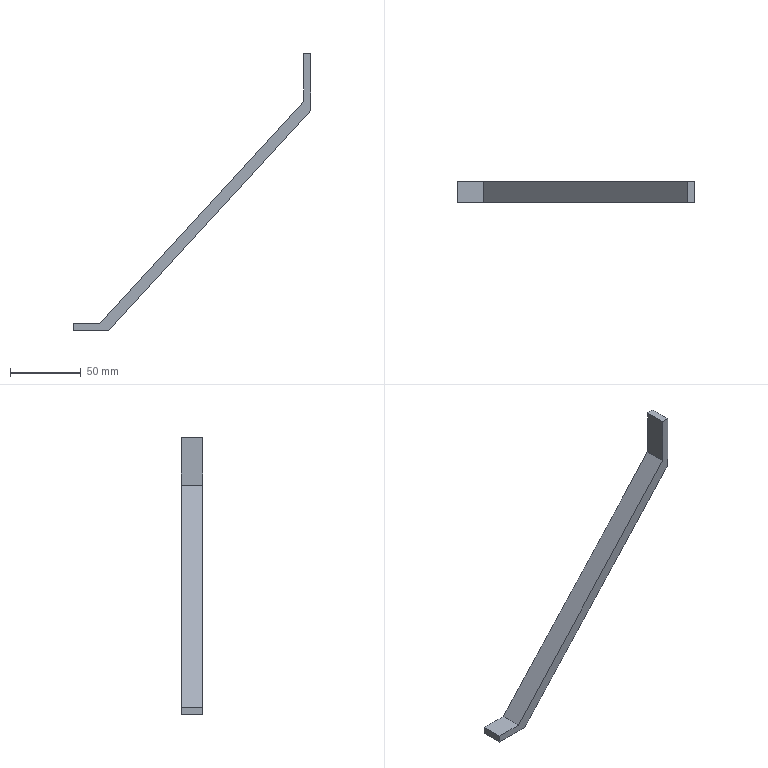Part | SolidWorks | features Extrusion 1 | 1 solid | 10 faces | box 167.5 x 15 x 195.2 mm | volume 29797 mm3 | plane 10
STEP:
#1=CARTESIAN_POINT('',(376.666,500.,456.3));
#2=VERTEX_POINT('',#1);
#3=CARTESIAN_POINT('',(371.666,500.,456.3));
#4=VERTEX_POINT('',#3);
#5=CARTESIAN_POINT('',(376.666,500.,456.3));
#6=DIRECTION('',(-1.,0.,0.));
#7=VECTOR('',#6,1000.);
#8=LINE('',#5,#7);
#9=EDGE_CURVE('',#2,#4,#8,.T.);
#10=ORIENTED_EDGE('',*,*,#9,.F.);
#11=CARTESIAN_POINT('',(376.666,515.,456.3));
#12=VERTEX_POINT('',#11);
#13=CARTESIAN_POINT('',(376.666,515.,456.3));
#14=DIRECTION('',(0.,-1.,0.));
#15=VECTOR('',#14,1000.);
#16=LINE('',#13,#15);
#17=EDGE_CURVE('',#12,#2,#16,.T.);
#18=ORIENTED_EDGE('',*,*,#17,.F.);
#19=CARTESIAN_POINT('',(371.666,515.,456.3));
#20=VERTEX_POINT('',#19);
#21=CARTESIAN_POINT('',(376.666,515.,456.3));
#22=DIRECTION('',(-1.,0.,0.));
#23=VECTOR('',#22,1000.);
#24=LINE('',#21,#23);
#25=EDGE_CURVE('',#12,#20,#24,.T.);
#26=ORIENTED_EDGE('',*,*,#25,.T.);
#27=CARTESIAN_POINT('',(371.666,515.,456.3));
#28=DIRECTION('',(0.,-1.,0.));
#29=VECTOR('',#28,1000.);
#30=LINE('',#27,#29);
#31=EDGE_CURVE('',#20,#4,#30,.T.);
#32=ORIENTED_EDGE('',*,*,#31,.T.);
#33=EDGE_LOOP('',(#10,#18,#26,#32));
#34=FACE_OUTER_BOUND('',#33,.T.);
#35=CARTESIAN_POINT('',(376.666,515.,456.3));
#36=DIRECTION('',(0.,0.,1.));
#37=DIRECTION('',(1.,0.,0.));
#38=AXIS2_PLACEMENT_3D('',#35,#36,#37);
#39=PLANE('',#38);
#40=ADVANCED_FACE('',(#34),#39,.T.);
#41=CARTESIAN_POINT('',(376.666,500.,416.3));
#42=VERTEX_POINT('',#41);
#43=CARTESIAN_POINT('',(376.666,500.,456.3));
#44=DIRECTION('',(0.,0.,1.));
#45=VECTOR('',#44,1000.);
#46=LINE('',#43,#45);
#47=EDGE_CURVE('',#42,#2,#46,.T.);
#48=ORIENTED_EDGE('',*,*,#47,.F.);
#49=CARTESIAN_POINT('',(376.666,515.,416.3));
#50=VERTEX_POINT('',#49);
#51=CARTESIAN_POINT('',(376.666,515.,416.3));
#52=DIRECTION('',(0.,-1.,0.));
#53=VECTOR('',#52,1000.);
#54=LINE('',#51,#53);
#55=EDGE_CURVE('',#50,#42,#54,.T.);
#56=ORIENTED_EDGE('',*,*,#55,.F.);
#57=CARTESIAN_POINT('',(376.666,515.,456.3));
#58=DIRECTION('',(0.,0.,1.));
#59=VECTOR('',#58,1000.);
#60=LINE('',#57,#59);
#61=EDGE_CURVE('',#50,#12,#60,.T.);
#62=ORIENTED_EDGE('',*,*,#61,.T.);
#63=ORIENTED_EDGE('',*,*,#17,.T.);
#64=EDGE_LOOP('',(#48,#56,#62,#63));
#65=FACE_OUTER_BOUND('',#64,.T.);
#66=CARTESIAN_POINT('',(376.666,515.,456.3));
#67=DIRECTION('',(1.,0.,0.));
#68=DIRECTION('',(0.,0.,-1.));
#69=AXIS2_PLACEMENT_3D('',#66,#67,#68);
#70=PLANE('',#69);
#71=ADVANCED_FACE('',(#65),#70,.T.);
#72=CARTESIAN_POINT('',(234.166,500.,261.1));
#73=VERTEX_POINT('',#72);
#74=CARTESIAN_POINT('',(376.666,500.,416.3));
#75=DIRECTION('',(0.6763,0.,0.7366));
#76=VECTOR('',#75,1000.);
#77=LINE('',#74,#76);
#78=EDGE_CURVE('',#73,#42,#77,.T.);
#79=ORIENTED_EDGE('',*,*,#78,.F.);
#80=CARTESIAN_POINT('',(234.166,515.,261.1));
#81=VERTEX_POINT('',#80);
#82=CARTESIAN_POINT('',(234.166,515.,261.1));
#83=DIRECTION('',(0.,-1.,0.));
#84=VECTOR('',#83,1000.);
#85=LINE('',#82,#84);
#86=EDGE_CURVE('',#81,#73,#85,.T.);
#87=ORIENTED_EDGE('',*,*,#86,.F.);
#88=CARTESIAN_POINT('',(376.666,515.,416.3));
#89=DIRECTION('',(0.6763,0.,0.7366));
#90=VECTOR('',#89,1000.);
#91=LINE('',#88,#90);
#92=EDGE_CURVE('',#81,#50,#91,.T.);
#93=ORIENTED_EDGE('',*,*,#92,.T.);
#94=ORIENTED_EDGE('',*,*,#55,.T.);
#95=EDGE_LOOP('',(#79,#87,#93,#94));
#96=FACE_OUTER_BOUND('',#95,.T.);
#97=CARTESIAN_POINT('',(376.666,515.,416.3));
#98=DIRECTION('',(0.7366,0.,-0.6763));
#99=DIRECTION('',(-0.6763,0.,-0.7366));
#100=AXIS2_PLACEMENT_3D('',#97,#98,#99);
#101=PLANE('',#100);
#102=ADVANCED_FACE('',(#96),#101,.T.);
#103=CARTESIAN_POINT('',(209.166,500.,261.1));
#104=VERTEX_POINT('',#103);
#105=CARTESIAN_POINT('',(209.166,500.,261.1));
#106=DIRECTION('',(1.,0.,0.));
#107=VECTOR('',#106,1000.);
#108=LINE('',#105,#107);
#109=EDGE_CURVE('',#104,#73,#108,.T.);
#110=ORIENTED_EDGE('',*,*,#109,.F.);
#111=CARTESIAN_POINT('',(209.166,515.,261.1));
#112=VERTEX_POINT('',#111);
#113=CARTESIAN_POINT('',(209.166,515.,261.1));
#114=DIRECTION('',(0.,-1.,0.));
#115=VECTOR('',#114,1000.);
#116=LINE('',#113,#115);
#117=EDGE_CURVE('',#112,#104,#116,.T.);
#118=ORIENTED_EDGE('',*,*,#117,.F.);
#119=CARTESIAN_POINT('',(209.166,515.,261.1));
#120=DIRECTION('',(1.,0.,0.));
#121=VECTOR('',#120,1000.);
#122=LINE('',#119,#121);
#123=EDGE_CURVE('',#112,#81,#122,.T.);
#124=ORIENTED_EDGE('',*,*,#123,.T.);
#125=ORIENTED_EDGE('',*,*,#86,.T.);
#126=EDGE_LOOP('',(#110,#118,#124,#125));
#127=FACE_OUTER_BOUND('',#126,.T.);
#128=CARTESIAN_POINT('',(209.166,515.,261.1));
#129=DIRECTION('',(0.,0.,-1.));
#130=DIRECTION('',(-1.,0.,0.));
#131=AXIS2_PLACEMENT_3D('',#128,#129,#130);
#132=PLANE('',#131);
#133=ADVANCED_FACE('',(#127),#132,.T.);
#134=CARTESIAN_POINT('',(209.166,500.,266.1));
#135=VERTEX_POINT('',#134);
#136=CARTESIAN_POINT('',(209.166,500.,261.1));
#137=DIRECTION('',(0.,0.,-1.));
#138=VECTOR('',#137,1000.);
#139=LINE('',#136,#138);
#140=EDGE_CURVE('',#135,#104,#139,.T.);
#141=ORIENTED_EDGE('',*,*,#140,.F.);
#142=CARTESIAN_POINT('',(209.166,515.,266.1));
#143=VERTEX_POINT('',#142);
#144=CARTESIAN_POINT('',(209.166,515.,266.1));
#145=DIRECTION('',(0.,-1.,0.));
#146=VECTOR('',#145,1000.);
#147=LINE('',#144,#146);
#148=EDGE_CURVE('',#143,#135,#147,.T.);
#149=ORIENTED_EDGE('',*,*,#148,.F.);
#150=CARTESIAN_POINT('',(209.166,515.,261.1));
#151=DIRECTION('',(0.,0.,-1.));
#152=VECTOR('',#151,1000.);
#153=LINE('',#150,#152);
#154=EDGE_CURVE('',#143,#112,#153,.T.);
#155=ORIENTED_EDGE('',*,*,#154,.T.);
#156=ORIENTED_EDGE('',*,*,#117,.T.);
#157=EDGE_LOOP('',(#141,#149,#155,#156));
#158=FACE_OUTER_BOUND('',#157,.T.);
#159=CARTESIAN_POINT('',(209.166,515.,261.1));
#160=DIRECTION('',(-1.,0.,0.));
#161=DIRECTION('',(0.,0.,1.));
#162=AXIS2_PLACEMENT_3D('',#159,#160,#161);
#163=PLANE('',#162);
#164=ADVANCED_FACE('',(#158),#163,.T.);
#165=CARTESIAN_POINT('',(227.897,500.,266.1));
#166=VERTEX_POINT('',#165);
#167=CARTESIAN_POINT('',(209.166,500.,266.1));
#168=DIRECTION('',(-1.,0.,0.));
#169=VECTOR('',#168,1000.);
#170=LINE('',#167,#169);
#171=EDGE_CURVE('',#166,#135,#170,.T.);
#172=ORIENTED_EDGE('',*,*,#171,.F.);
#173=CARTESIAN_POINT('',(227.897,515.,266.1));
#174=VERTEX_POINT('',#173);
#175=CARTESIAN_POINT('',(227.897,515.,266.1));
#176=DIRECTION('',(0.,-1.,0.));
#177=VECTOR('',#176,1000.);
#178=LINE('',#175,#177);
#179=EDGE_CURVE('',#174,#166,#178,.T.);
#180=ORIENTED_EDGE('',*,*,#179,.F.);
#181=CARTESIAN_POINT('',(209.166,515.,266.1));
#182=DIRECTION('',(-1.,0.,0.));
#183=VECTOR('',#182,1000.);
#184=LINE('',#181,#183);
#185=EDGE_CURVE('',#174,#143,#184,.T.);
#186=ORIENTED_EDGE('',*,*,#185,.T.);
#187=ORIENTED_EDGE('',*,*,#148,.T.);
#188=EDGE_LOOP('',(#172,#180,#186,#187));
#189=FACE_OUTER_BOUND('',#188,.T.);
#190=CARTESIAN_POINT('',(209.166,515.,266.1));
#191=DIRECTION('',(0.,0.,1.));
#192=DIRECTION('',(1.,0.,0.));
#193=AXIS2_PLACEMENT_3D('',#190,#191,#192);
#194=PLANE('',#193);
#195=ADVANCED_FACE('',(#189),#194,.T.);
#196=CARTESIAN_POINT('',(371.666,500.,422.683));
#197=VERTEX_POINT('',#196);
#198=CARTESIAN_POINT('',(361.871,500.,412.014));
#199=DIRECTION('',(-0.6763,0.,-0.7366));
#200=VECTOR('',#199,1000.);
#201=LINE('',#198,#200);
#202=EDGE_CURVE('',#197,#166,#201,.T.);
#203=ORIENTED_EDGE('',*,*,#202,.F.);
#204=CARTESIAN_POINT('',(371.666,515.,422.683));
#205=VERTEX_POINT('',#204);
#206=CARTESIAN_POINT('',(371.666,515.,422.683));
#207=DIRECTION('',(0.,-1.,0.));
#208=VECTOR('',#207,1000.);
#209=LINE('',#206,#208);
#210=EDGE_CURVE('',#205,#197,#209,.T.);
#211=ORIENTED_EDGE('',*,*,#210,.F.);
#212=CARTESIAN_POINT('',(361.871,515.,412.014));
#213=DIRECTION('',(-0.6763,0.,-0.7366));
#214=VECTOR('',#213,1000.);
#215=LINE('',#212,#214);
#216=EDGE_CURVE('',#205,#174,#215,.T.);
#217=ORIENTED_EDGE('',*,*,#216,.T.);
#218=ORIENTED_EDGE('',*,*,#179,.T.);
#219=EDGE_LOOP('',(#203,#211,#217,#218));
#220=FACE_OUTER_BOUND('',#219,.T.);
#221=CARTESIAN_POINT('',(361.871,515.,412.014));
#222=DIRECTION('',(-0.7366,0.,0.6763));
#223=DIRECTION('',(0.6763,0.,0.7366));
#224=AXIS2_PLACEMENT_3D('',#221,#222,#223);
#225=PLANE('',#224);
#226=ADVANCED_FACE('',(#220),#225,.T.);
#227=CARTESIAN_POINT('',(371.666,500.,456.3));
#228=DIRECTION('',(0.,0.,-1.));
#229=VECTOR('',#228,1000.);
#230=LINE('',#227,#229);
#231=EDGE_CURVE('',#4,#197,#230,.T.);
#232=ORIENTED_EDGE('',*,*,#231,.F.);
#233=ORIENTED_EDGE('',*,*,#31,.F.);
#234=CARTESIAN_POINT('',(371.666,515.,456.3));
#235=DIRECTION('',(0.,0.,-1.));
#236=VECTOR('',#235,1000.);
#237=LINE('',#234,#236);
#238=EDGE_CURVE('',#20,#205,#237,.T.);
#239=ORIENTED_EDGE('',*,*,#238,.T.);
#240=ORIENTED_EDGE('',*,*,#210,.T.);
#241=EDGE_LOOP('',(#232,#233,#239,#240));
#242=FACE_OUTER_BOUND('',#241,.T.);
#243=CARTESIAN_POINT('',(371.666,515.,456.3));
#244=DIRECTION('',(-1.,0.,0.));
#245=DIRECTION('',(0.,0.,1.));
#246=AXIS2_PLACEMENT_3D('',#243,#244,#245);
#247=PLANE('',#246);
#248=ADVANCED_FACE('',(#242),#247,.T.);
#249=ORIENTED_EDGE('',*,*,#25,.F.);
#250=ORIENTED_EDGE('',*,*,#61,.F.);
#251=ORIENTED_EDGE('',*,*,#92,.F.);
#252=ORIENTED_EDGE('',*,*,#123,.F.);
#253=ORIENTED_EDGE('',*,*,#154,.F.);
#254=ORIENTED_EDGE('',*,*,#185,.F.);
#255=ORIENTED_EDGE('',*,*,#216,.F.);
#256=ORIENTED_EDGE('',*,*,#238,.F.);
#257=EDGE_LOOP('',(#249,#250,#251,#252,#253,#254,#255,#256));
#258=FACE_OUTER_BOUND('',#257,.T.);
#259=CARTESIAN_POINT('',(0.,515.,0.));
#260=DIRECTION('',(0.,-1.,0.));
#261=DIRECTION('',(0.,0.,-1.));
#262=AXIS2_PLACEMENT_3D('',#259,#260,#261);
#263=PLANE('',#262);
#264=ADVANCED_FACE('',(#258),#263,.F.);
#265=ORIENTED_EDGE('',*,*,#9,.T.);
#266=ORIENTED_EDGE('',*,*,#231,.T.);
#267=ORIENTED_EDGE('',*,*,#202,.T.);
#268=ORIENTED_EDGE('',*,*,#171,.T.);
#269=ORIENTED_EDGE('',*,*,#140,.T.);
#270=ORIENTED_EDGE('',*,*,#109,.T.);
#271=ORIENTED_EDGE('',*,*,#78,.T.);
#272=ORIENTED_EDGE('',*,*,#47,.T.);
#273=EDGE_LOOP('',(#265,#266,#267,#268,#269,#270,#271,#272));
#274=FACE_OUTER_BOUND('',#273,.T.);
#275=CARTESIAN_POINT('',(0.,500.,0.));
#276=DIRECTION('',(0.,-1.,0.));
#277=DIRECTION('',(0.,0.,-1.));
#278=AXIS2_PLACEMENT_3D('',#275,#276,#277);
#279=PLANE('',#278);
#280=ADVANCED_FACE('',(#274),#279,.T.);
#281=CLOSED_SHELL('',(#40,#71,#102,#133,#164,#195,#226,#248,#264,#280));
#282=MANIFOLD_SOLID_BREP('',#281);
#283=CARTESIAN_POINT('',(0.,0.,0.));
#284=DIRECTION('',(0.,0.,1.));
#285=DIRECTION('',(1.,0.,0.));
#286=AXIS2_PLACEMENT_3D('',#283,#284,#285);
#287=(LENGTH_UNIT()NAMED_UNIT(*)SI_UNIT(.MILLI.,.METRE.));
#288=UNCERTAINTY_MEASURE_WITH_UNIT(LENGTH_MEASURE(0.00001),#287,'','');
#289=(NAMED_UNIT(*)PLANE_ANGLE_UNIT()SI_UNIT($,.RADIAN.));
#290=(NAMED_UNIT(*)SI_UNIT($,.STERADIAN.)SOLID_ANGLE_UNIT());
#291=(GEOMETRIC_REPRESENTATION_CONTEXT(3)GLOBAL_UNCERTAINTY_ASSIGNED_CONTEXT((#288))GLOBAL_UNIT_ASSIGNED_CONTEXT((#287,#289,#290))REPRESENTATION_CONTEXT('',''));
#292=ADVANCED_BREP_SHAPE_REPRESENTATION('',(#282,#286),#291);